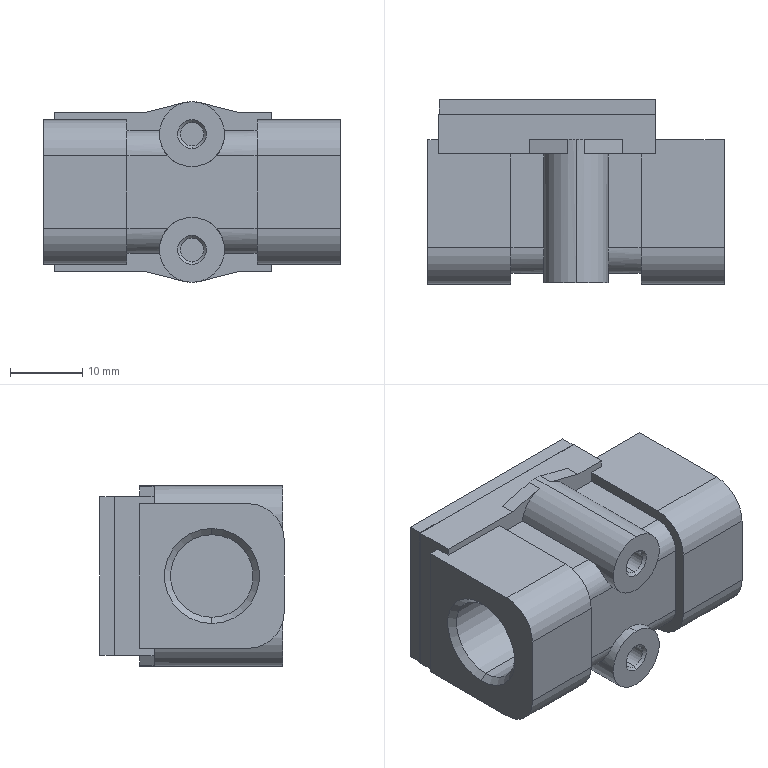Part | SolidWorks | features BaseBody 1 | 1 solid | 71 faces | box 41 x 25.5 x 25 mm | volume 17055 mm3 | plane 43 | cylinder 20 | cone 8 | commonest cylinder face diameters 3.242 x4 7 x4 9 x4 10 x4 11.445 x4